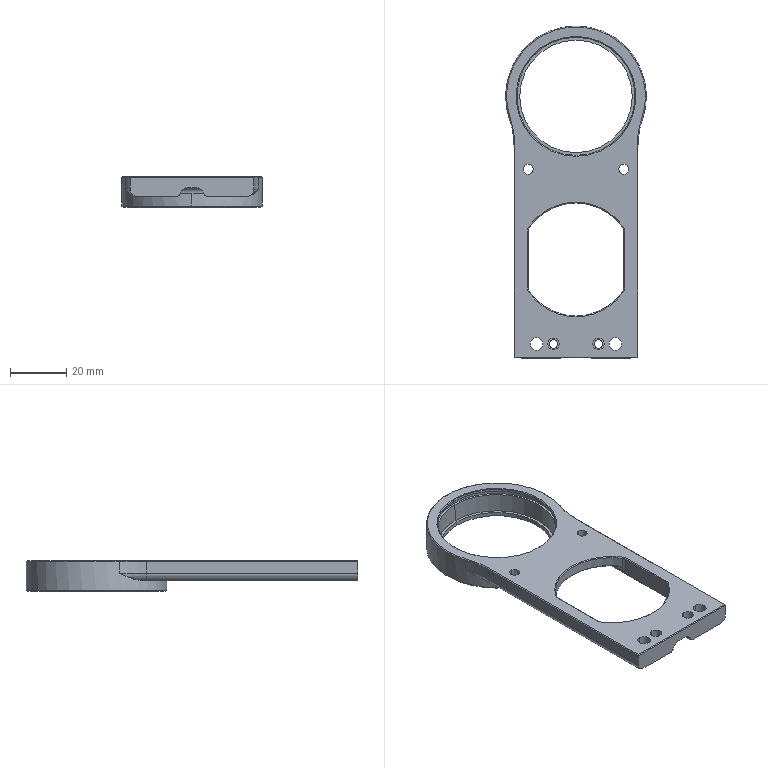NC program | NX | posted with a generic post | part box 50 x 118 x 11 mm
Lines 1 to 18 of 3723:
N10 G17 G21 G94 G90
(FLOOR_WALL , TOOL : D80)
N12 T19 M6
N14 G54
N16 G17 G0 G90 X-104. Y0. S5000 M3
N18 G43 Z30. H19
N20 Z3.
N22 G94 G1 Z0. F1200.
N24 X-101.
N26 X101.
N28 X104.
N30 Z3.
N32 G0 Z30.
N34 M5